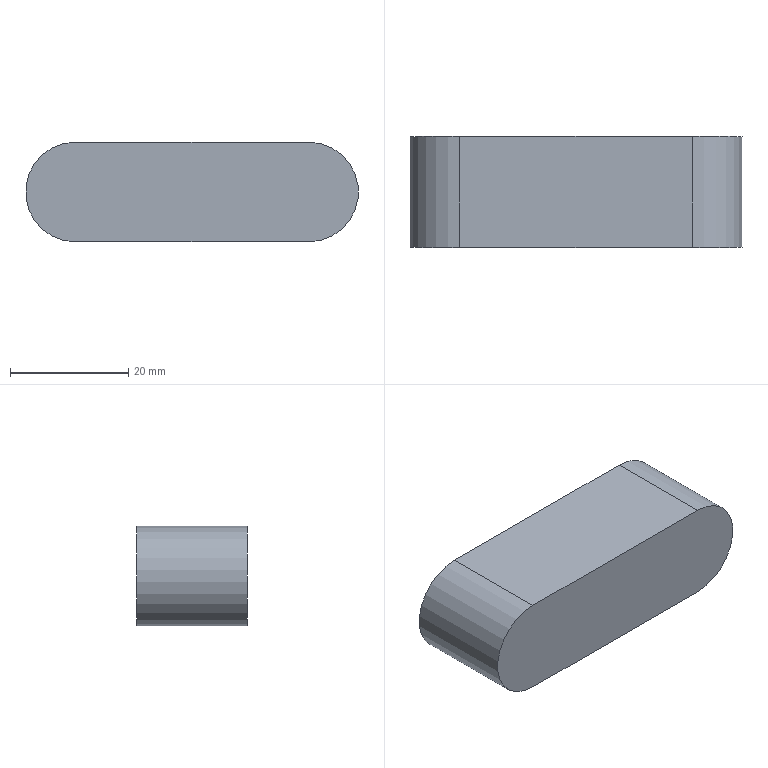Part | SolidWorks | features Extrusion 1, Scale 1 | 1 solid | 6 faces | box 56.25 x 18.75 x 16.875 mm | volume 16652 mm3 | plane 4 | cylinder 2 | commonest cylinder face diameters 16.875 x2
STEP:
#1=CARTESIAN_POINT('',(-9.188,-4.375,-8.437));
#2=VERTEX_POINT('',#1);
#3=CARTESIAN_POINT('',(-9.188,-4.375,8.437));
#4=VERTEX_POINT('',#3);
#5=CARTESIAN_POINT('',(-9.188,-4.375,0.));
#6=DIRECTION('',(0.,1.,0.));
#7=DIRECTION('',(0.,0.,1.));
#8=AXIS2_PLACEMENT_3D('',#5,#6,#7);
#9=CIRCLE('',#8,8.437);
#10=EDGE_CURVE('',#2,#4,#9,.T.);
#11=ORIENTED_EDGE('',*,*,#10,.T.);
#12=CARTESIAN_POINT('',(-9.188,14.375,8.437));
#13=VERTEX_POINT('',#12);
#14=CARTESIAN_POINT('',(-9.188,14.375,8.437));
#15=DIRECTION('',(0.,-1.,0.));
#16=VECTOR('',#15,1000.);
#17=LINE('',#14,#16);
#18=EDGE_CURVE('',#13,#4,#17,.T.);
#19=ORIENTED_EDGE('',*,*,#18,.F.);
#20=CARTESIAN_POINT('',(-9.188,14.375,-8.437));
#21=VERTEX_POINT('',#20);
#22=CARTESIAN_POINT('',(-9.188,14.375,0.));
#23=DIRECTION('',(0.,1.,0.));
#24=DIRECTION('',(0.,0.,1.));
#25=AXIS2_PLACEMENT_3D('',#22,#23,#24);
#26=CIRCLE('',#25,8.437);
#27=EDGE_CURVE('',#21,#13,#26,.T.);
#28=ORIENTED_EDGE('',*,*,#27,.F.);
#29=CARTESIAN_POINT('',(-9.188,14.375,-8.437));
#30=DIRECTION('',(0.,-1.,0.));
#31=VECTOR('',#30,1000.);
#32=LINE('',#29,#31);
#33=EDGE_CURVE('',#21,#2,#32,.T.);
#34=ORIENTED_EDGE('',*,*,#33,.T.);
#35=EDGE_LOOP('',(#11,#19,#28,#34));
#36=FACE_OUTER_BOUND('',#35,.T.);
#37=CARTESIAN_POINT('',(-9.188,14.375,0.));
#38=DIRECTION('',(0.,-1.,0.));
#39=DIRECTION('',(0.,0.,-1.));
#40=AXIS2_PLACEMENT_3D('',#37,#38,#39);
#41=CYLINDRICAL_SURFACE('',#40,8.437);
#42=ADVANCED_FACE('',(#36),#41,.T.);
#43=CARTESIAN_POINT('',(30.188,-4.375,8.437));
#44=VERTEX_POINT('',#43);
#45=CARTESIAN_POINT('',(-9.188,-4.375,8.437));
#46=DIRECTION('',(1.,0.,0.));
#47=VECTOR('',#46,1000.);
#48=LINE('',#45,#47);
#49=EDGE_CURVE('',#4,#44,#48,.T.);
#50=ORIENTED_EDGE('',*,*,#49,.T.);
#51=CARTESIAN_POINT('',(30.188,14.375,8.437));
#52=VERTEX_POINT('',#51);
#53=CARTESIAN_POINT('',(30.188,14.375,8.437));
#54=DIRECTION('',(0.,-1.,0.));
#55=VECTOR('',#54,1000.);
#56=LINE('',#53,#55);
#57=EDGE_CURVE('',#52,#44,#56,.T.);
#58=ORIENTED_EDGE('',*,*,#57,.F.);
#59=CARTESIAN_POINT('',(-9.188,14.375,8.437));
#60=DIRECTION('',(1.,0.,0.));
#61=VECTOR('',#60,1000.);
#62=LINE('',#59,#61);
#63=EDGE_CURVE('',#13,#52,#62,.T.);
#64=ORIENTED_EDGE('',*,*,#63,.F.);
#65=ORIENTED_EDGE('',*,*,#18,.T.);
#66=EDGE_LOOP('',(#50,#58,#64,#65));
#67=FACE_OUTER_BOUND('',#66,.T.);
#68=CARTESIAN_POINT('',(-9.188,14.375,8.437));
#69=DIRECTION('',(0.,0.,-1.));
#70=DIRECTION('',(-1.,0.,0.));
#71=AXIS2_PLACEMENT_3D('',#68,#69,#70);
#72=PLANE('',#71);
#73=ADVANCED_FACE('',(#67),#72,.F.);
#74=CARTESIAN_POINT('',(30.188,-4.375,-8.437));
#75=VERTEX_POINT('',#74);
#76=CARTESIAN_POINT('',(30.188,-4.375,0.));
#77=DIRECTION('',(0.,1.,0.));
#78=DIRECTION('',(0.,0.,1.));
#79=AXIS2_PLACEMENT_3D('',#76,#77,#78);
#80=CIRCLE('',#79,8.437);
#81=EDGE_CURVE('',#44,#75,#80,.T.);
#82=ORIENTED_EDGE('',*,*,#81,.T.);
#83=CARTESIAN_POINT('',(30.188,14.375,-8.437));
#84=VERTEX_POINT('',#83);
#85=CARTESIAN_POINT('',(30.188,14.375,-8.437));
#86=DIRECTION('',(0.,-1.,0.));
#87=VECTOR('',#86,1000.);
#88=LINE('',#85,#87);
#89=EDGE_CURVE('',#84,#75,#88,.T.);
#90=ORIENTED_EDGE('',*,*,#89,.F.);
#91=CARTESIAN_POINT('',(30.188,14.375,0.));
#92=DIRECTION('',(0.,1.,0.));
#93=DIRECTION('',(0.,0.,1.));
#94=AXIS2_PLACEMENT_3D('',#91,#92,#93);
#95=CIRCLE('',#94,8.437);
#96=EDGE_CURVE('',#52,#84,#95,.T.);
#97=ORIENTED_EDGE('',*,*,#96,.F.);
#98=ORIENTED_EDGE('',*,*,#57,.T.);
#99=EDGE_LOOP('',(#82,#90,#97,#98));
#100=FACE_OUTER_BOUND('',#99,.T.);
#101=CARTESIAN_POINT('',(30.188,14.375,0.));
#102=DIRECTION('',(0.,-1.,0.));
#103=DIRECTION('',(0.,0.,-1.));
#104=AXIS2_PLACEMENT_3D('',#101,#102,#103);
#105=CYLINDRICAL_SURFACE('',#104,8.437);
#106=ADVANCED_FACE('',(#100),#105,.T.);
#107=CARTESIAN_POINT('',(-9.188,-4.375,-8.437));
#108=DIRECTION('',(-1.,0.,0.));
#109=VECTOR('',#108,1000.);
#110=LINE('',#107,#109);
#111=EDGE_CURVE('',#75,#2,#110,.T.);
#112=ORIENTED_EDGE('',*,*,#111,.T.);
#113=ORIENTED_EDGE('',*,*,#33,.F.);
#114=CARTESIAN_POINT('',(-9.188,14.375,-8.437));
#115=DIRECTION('',(-1.,0.,0.));
#116=VECTOR('',#115,1000.);
#117=LINE('',#114,#116);
#118=EDGE_CURVE('',#84,#21,#117,.T.);
#119=ORIENTED_EDGE('',*,*,#118,.F.);
#120=ORIENTED_EDGE('',*,*,#89,.T.);
#121=EDGE_LOOP('',(#112,#113,#119,#120));
#122=FACE_OUTER_BOUND('',#121,.T.);
#123=CARTESIAN_POINT('',(-9.188,14.375,-8.437));
#124=DIRECTION('',(0.,0.,1.));
#125=DIRECTION('',(1.,0.,0.));
#126=AXIS2_PLACEMENT_3D('',#123,#124,#125);
#127=PLANE('',#126);
#128=ADVANCED_FACE('',(#122),#127,.F.);
#129=ORIENTED_EDGE('',*,*,#27,.T.);
#130=ORIENTED_EDGE('',*,*,#63,.T.);
#131=ORIENTED_EDGE('',*,*,#96,.T.);
#132=ORIENTED_EDGE('',*,*,#118,.T.);
#133=EDGE_LOOP('',(#129,#130,#131,#132));
#134=FACE_OUTER_BOUND('',#133,.T.);
#135=CARTESIAN_POINT('',(-9.188,14.375,0.));
#136=DIRECTION('',(0.,1.,0.));
#137=DIRECTION('',(0.,0.,1.));
#138=AXIS2_PLACEMENT_3D('',#135,#136,#137);
#139=PLANE('',#138);
#140=ADVANCED_FACE('',(#134),#139,.T.);
#141=ORIENTED_EDGE('',*,*,#10,.F.);
#142=ORIENTED_EDGE('',*,*,#111,.F.);
#143=ORIENTED_EDGE('',*,*,#81,.F.);
#144=ORIENTED_EDGE('',*,*,#49,.F.);
#145=EDGE_LOOP('',(#141,#142,#143,#144));
#146=FACE_OUTER_BOUND('',#145,.T.);
#147=CARTESIAN_POINT('',(-9.188,-4.375,0.));
#148=DIRECTION('',(0.,1.,0.));
#149=DIRECTION('',(0.,0.,1.));
#150=AXIS2_PLACEMENT_3D('',#147,#148,#149);
#151=PLANE('',#150);
#152=ADVANCED_FACE('',(#146),#151,.F.);
#153=CLOSED_SHELL('',(#42,#73,#106,#128,#140,#152));
#154=MANIFOLD_SOLID_BREP('',#153);
#155=CARTESIAN_POINT('',(0.,0.,0.));
#156=DIRECTION('',(0.,0.,1.));
#157=DIRECTION('',(1.,0.,0.));
#158=AXIS2_PLACEMENT_3D('',#155,#156,#157);
#159=(LENGTH_UNIT()NAMED_UNIT(*)SI_UNIT(.MILLI.,.METRE.));
#160=UNCERTAINTY_MEASURE_WITH_UNIT(LENGTH_MEASURE(0.00001),#159,'','');
#161=(NAMED_UNIT(*)PLANE_ANGLE_UNIT()SI_UNIT($,.RADIAN.));
#162=(NAMED_UNIT(*)SI_UNIT($,.STERADIAN.)SOLID_ANGLE_UNIT());
#163=(GEOMETRIC_REPRESENTATION_CONTEXT(3)GLOBAL_UNCERTAINTY_ASSIGNED_CONTEXT((#160))GLOBAL_UNIT_ASSIGNED_CONTEXT((#159,#161,#162))REPRESENTATION_CONTEXT('',''));
#164=ADVANCED_BREP_SHAPE_REPRESENTATION('',(#154,#158),#163);